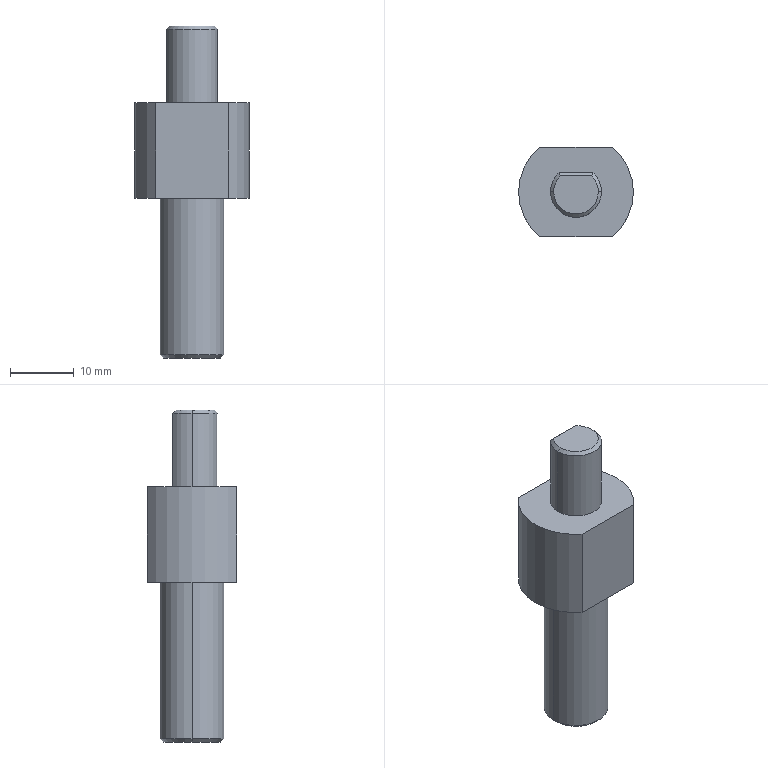Part | SolidWorks | features ICE 2, Chamfer 1, Extrusion 1 | 1 solid | 21 faces | box 18 x 14 x 52 mm | volume 5870 mm3 | cylinder 8 | plane 8 | cone 5 | commonest cylinder face diameters 8 x3 18 x3 10 x2
STEP:
#1=CARTESIAN_POINT('',(-4.5,0.,-52.));
#2=VERTEX_POINT('',#1);
#3=CARTESIAN_POINT('',(4.5,0.,-52.));
#4=VERTEX_POINT('',#3);
#5=CARTESIAN_POINT('',(0.,0.,-52.));
#6=DIRECTION('',(0.,0.,-1.));
#7=DIRECTION('',(-1.,0.,0.));
#8=AXIS2_PLACEMENT_3D('',#5,#6,#7);
#9=CIRCLE('',#8,4.5);
#10=EDGE_CURVE('',#2,#4,#9,.T.);
#11=ORIENTED_EDGE('',*,*,#10,.F.);
#12=CARTESIAN_POINT('',(-5.,0.,-51.5));
#13=VERTEX_POINT('',#12);
#14=CARTESIAN_POINT('',(-4.5,0.,-52.));
#15=DIRECTION('',(-0.7071,0.,0.7071));
#16=VECTOR('',#15,1000.);
#17=LINE('',#14,#16);
#18=EDGE_CURVE('',#2,#13,#17,.T.);
#19=ORIENTED_EDGE('',*,*,#18,.T.);
#20=CARTESIAN_POINT('',(5.,0.,-51.5));
#21=VERTEX_POINT('',#20);
#22=CARTESIAN_POINT('',(0.,0.,-51.5));
#23=DIRECTION('',(0.,0.,1.));
#24=DIRECTION('',(-1.,0.,0.));
#25=AXIS2_PLACEMENT_3D('',#22,#23,#24);
#26=CIRCLE('',#25,5.);
#27=EDGE_CURVE('',#21,#13,#26,.T.);
#28=ORIENTED_EDGE('',*,*,#27,.F.);
#29=CARTESIAN_POINT('',(4.5,0.,-52.));
#30=DIRECTION('',(0.7071,0.,0.7071));
#31=VECTOR('',#30,1000.);
#32=LINE('',#29,#31);
#33=EDGE_CURVE('',#4,#21,#32,.T.);
#34=ORIENTED_EDGE('',*,*,#33,.F.);
#35=EDGE_LOOP('',(#11,#19,#28,#34));
#36=FACE_OUTER_BOUND('',#35,.T.);
#37=CARTESIAN_POINT('',(0.,0.,-52.));
#38=DIRECTION('',(0.,0.,1.));
#39=DIRECTION('',(1.,0.,0.));
#40=AXIS2_PLACEMENT_3D('',#37,#38,#39);
#41=CONICAL_SURFACE('',#40,4.5,0.7854);
#42=ADVANCED_FACE('',(#36),#41,.T.);
#43=CARTESIAN_POINT('',(3.5,0.,0.));
#44=VERTEX_POINT('',#43);
#45=CARTESIAN_POINT('',(2.449,2.5,0.));
#46=VERTEX_POINT('',#45);
#47=CARTESIAN_POINT('',(0.,0.,0.));
#48=DIRECTION('',(0.,0.,1.));
#49=DIRECTION('',(1.,0.,0.));
#50=AXIS2_PLACEMENT_3D('',#47,#48,#49);
#51=CIRCLE('',#50,3.5);
#52=EDGE_CURVE('',#44,#46,#51,.T.);
#53=ORIENTED_EDGE('',*,*,#52,.F.);
#54=CARTESIAN_POINT('',(4.,0.,-0.5));
#55=VERTEX_POINT('',#54);
#56=CARTESIAN_POINT('',(3.5,0.,0.));
#57=DIRECTION('',(0.7071,0.,-0.7071));
#58=VECTOR('',#57,1000.);
#59=LINE('',#56,#58);
#60=EDGE_CURVE('',#44,#55,#59,.T.);
#61=ORIENTED_EDGE('',*,*,#60,.T.);
#62=CARTESIAN_POINT('',(2.646,3.,-0.5));
#63=VERTEX_POINT('',#62);
#64=CARTESIAN_POINT('',(0.,0.,-0.5));
#65=DIRECTION('',(0.,0.,-1.));
#66=DIRECTION('',(1.,0.,0.));
#67=AXIS2_PLACEMENT_3D('',#64,#65,#66);
#68=CIRCLE('',#67,4.);
#69=EDGE_CURVE('',#63,#55,#68,.T.);
#70=ORIENTED_EDGE('',*,*,#69,.F.);
#71=CARTESIAN_POINT('',(2.449,2.5,0.));
#72=CARTESIAN_POINT('',(2.517,2.666,-0.1662));
#73=CARTESIAN_POINT('',(2.583,2.833,-0.3329));
#74=CARTESIAN_POINT('',(2.646,3.,-0.5));
#75=B_SPLINE_CURVE_WITH_KNOTS('',3,(#71,#72,#73,#74),.UNSPECIFIED.,.F.,.F.,(4,4),(0.,0.0007338),.UNSPECIFIED.);
#76=EDGE_CURVE('',#46,#63,#75,.T.);
#77=ORIENTED_EDGE('',*,*,#76,.F.);
#78=EDGE_LOOP('',(#53,#61,#70,#77));
#79=FACE_OUTER_BOUND('',#78,.T.);
#80=CARTESIAN_POINT('',(0.,0.,0.));
#81=DIRECTION('',(0.,0.,-1.));
#82=DIRECTION('',(-1.,0.,0.));
#83=AXIS2_PLACEMENT_3D('',#80,#81,#82);
#84=CONICAL_SURFACE('',#83,3.5,0.7854);
#85=ADVANCED_FACE('',(#79),#84,.T.);
#86=ORIENTED_EDGE('',*,*,#60,.F.);
#87=CARTESIAN_POINT('',(-3.5,0.,0.));
#88=VERTEX_POINT('',#87);
#89=CARTESIAN_POINT('',(0.,0.,0.));
#90=DIRECTION('',(0.,0.,1.));
#91=DIRECTION('',(1.,0.,0.));
#92=AXIS2_PLACEMENT_3D('',#89,#90,#91);
#93=CIRCLE('',#92,3.5);
#94=EDGE_CURVE('',#88,#44,#93,.T.);
#95=ORIENTED_EDGE('',*,*,#94,.F.);
#96=CARTESIAN_POINT('',(-4.,0.,-0.5));
#97=VERTEX_POINT('',#96);
#98=CARTESIAN_POINT('',(-3.5,0.,0.));
#99=DIRECTION('',(-0.7071,0.,-0.7071));
#100=VECTOR('',#99,1000.);
#101=LINE('',#98,#100);
#102=EDGE_CURVE('',#88,#97,#101,.T.);
#103=ORIENTED_EDGE('',*,*,#102,.T.);
#104=CARTESIAN_POINT('',(0.,0.,-0.5));
#105=DIRECTION('',(0.,0.,-1.));
#106=DIRECTION('',(1.,0.,0.));
#107=AXIS2_PLACEMENT_3D('',#104,#105,#106);
#108=CIRCLE('',#107,4.);
#109=EDGE_CURVE('',#55,#97,#108,.T.);
#110=ORIENTED_EDGE('',*,*,#109,.F.);
#111=EDGE_LOOP('',(#86,#95,#103,#110));
#112=FACE_OUTER_BOUND('',#111,.T.);
#113=CARTESIAN_POINT('',(0.,0.,0.));
#114=DIRECTION('',(0.,0.,-1.));
#115=DIRECTION('',(-1.,0.,0.));
#116=AXIS2_PLACEMENT_3D('',#113,#114,#115);
#117=CONICAL_SURFACE('',#116,3.5,0.7854);
#118=ADVANCED_FACE('',(#112),#117,.T.);
#119=ORIENTED_EDGE('',*,*,#27,.T.);
#120=CARTESIAN_POINT('',(-5.,0.,-27.));
#121=VERTEX_POINT('',#120);
#122=CARTESIAN_POINT('',(-5.,0.,-52.));
#123=DIRECTION('',(0.,0.,1.));
#124=VECTOR('',#123,1000.);
#125=LINE('',#122,#124);
#126=EDGE_CURVE('',#13,#121,#125,.T.);
#127=ORIENTED_EDGE('',*,*,#126,.T.);
#128=CARTESIAN_POINT('',(5.,0.,-27.));
#129=VERTEX_POINT('',#128);
#130=CARTESIAN_POINT('',(0.,0.,-27.));
#131=DIRECTION('',(0.,0.,-1.));
#132=DIRECTION('',(-1.,0.,0.));
#133=AXIS2_PLACEMENT_3D('',#130,#131,#132);
#134=CIRCLE('',#133,5.);
#135=EDGE_CURVE('',#121,#129,#134,.T.);
#136=ORIENTED_EDGE('',*,*,#135,.T.);
#137=CARTESIAN_POINT('',(5.,0.,-52.));
#138=DIRECTION('',(0.,0.,1.));
#139=VECTOR('',#138,1000.);
#140=LINE('',#137,#139);
#141=EDGE_CURVE('',#21,#129,#140,.T.);
#142=ORIENTED_EDGE('',*,*,#141,.F.);
#143=EDGE_LOOP('',(#119,#127,#136,#142));
#144=FACE_OUTER_BOUND('',#143,.T.);
#145=CARTESIAN_POINT('',(0.,0.,-52.));
#146=DIRECTION('',(0.,0.,1.));
#147=DIRECTION('',(1.,0.,0.));
#148=AXIS2_PLACEMENT_3D('',#145,#146,#147);
#149=CYLINDRICAL_SURFACE('',#148,5.);
#150=ADVANCED_FACE('',(#144),#149,.T.);
#151=CARTESIAN_POINT('',(9.,0.,-27.));
#152=VERTEX_POINT('',#151);
#153=CARTESIAN_POINT('',(5.657,-7.,-27.));
#154=VERTEX_POINT('',#153);
#155=CARTESIAN_POINT('',(0.,0.,-27.));
#156=DIRECTION('',(0.,0.,-1.));
#157=DIRECTION('',(-1.,0.,0.));
#158=AXIS2_PLACEMENT_3D('',#155,#156,#157);
#159=CIRCLE('',#158,9.);
#160=EDGE_CURVE('',#152,#154,#159,.T.);
#161=ORIENTED_EDGE('',*,*,#160,.F.);
#162=CARTESIAN_POINT('',(9.,0.,-12.));
#163=VERTEX_POINT('',#162);
#164=CARTESIAN_POINT('',(9.,0.,-27.));
#165=DIRECTION('',(0.,0.,1.));
#166=VECTOR('',#165,1000.);
#167=LINE('',#164,#166);
#168=EDGE_CURVE('',#152,#163,#167,.T.);
#169=ORIENTED_EDGE('',*,*,#168,.T.);
#170=CARTESIAN_POINT('',(5.657,-7.,-12.));
#171=VERTEX_POINT('',#170);
#172=CARTESIAN_POINT('',(0.,0.,-12.));
#173=DIRECTION('',(0.,0.,-1.));
#174=DIRECTION('',(-1.,0.,0.));
#175=AXIS2_PLACEMENT_3D('',#172,#173,#174);
#176=CIRCLE('',#175,9.);
#177=EDGE_CURVE('',#163,#171,#176,.T.);
#178=ORIENTED_EDGE('',*,*,#177,.T.);
#179=CARTESIAN_POINT('',(5.657,-7.,-27.));
#180=DIRECTION('',(0.,0.,1.));
#181=VECTOR('',#180,1000.);
#182=LINE('',#179,#181);
#183=EDGE_CURVE('',#154,#171,#182,.T.);
#184=ORIENTED_EDGE('',*,*,#183,.F.);
#185=EDGE_LOOP('',(#161,#169,#178,#184));
#186=FACE_OUTER_BOUND('',#185,.T.);
#187=CARTESIAN_POINT('',(0.,0.,-27.));
#188=DIRECTION('',(0.,0.,1.));
#189=DIRECTION('',(1.,0.,0.));
#190=AXIS2_PLACEMENT_3D('',#187,#188,#189);
#191=CYLINDRICAL_SURFACE('',#190,9.);
#192=ADVANCED_FACE('',(#186),#191,.T.);
#193=CARTESIAN_POINT('',(-2.646,3.,-12.));
#194=VERTEX_POINT('',#193);
#195=CARTESIAN_POINT('',(-4.,0.,-12.));
#196=VERTEX_POINT('',#195);
#197=CARTESIAN_POINT('',(0.,0.,-12.));
#198=DIRECTION('',(0.,0.,1.));
#199=DIRECTION('',(1.,0.,0.));
#200=AXIS2_PLACEMENT_3D('',#197,#198,#199);
#201=CIRCLE('',#200,4.);
#202=EDGE_CURVE('',#194,#196,#201,.T.);
#203=ORIENTED_EDGE('',*,*,#202,.T.);
#204=CARTESIAN_POINT('',(-4.,0.,-12.));
#205=DIRECTION('',(0.,0.,1.));
#206=VECTOR('',#205,1000.);
#207=LINE('',#204,#206);
#208=EDGE_CURVE('',#196,#97,#207,.T.);
#209=ORIENTED_EDGE('',*,*,#208,.T.);
#210=CARTESIAN_POINT('',(-2.646,3.,-0.5));
#211=VERTEX_POINT('',#210);
#212=CARTESIAN_POINT('',(0.,0.,-0.5));
#213=DIRECTION('',(0.,0.,-1.));
#214=DIRECTION('',(1.,0.,0.));
#215=AXIS2_PLACEMENT_3D('',#212,#213,#214);
#216=CIRCLE('',#215,4.);
#217=EDGE_CURVE('',#97,#211,#216,.T.);
#218=ORIENTED_EDGE('',*,*,#217,.T.);
#219=CARTESIAN_POINT('',(-2.646,3.,-12.));
#220=DIRECTION('',(0.,0.,1.));
#221=VECTOR('',#220,1000.);
#222=LINE('',#219,#221);
#223=EDGE_CURVE('',#194,#211,#222,.T.);
#224=ORIENTED_EDGE('',*,*,#223,.F.);
#225=EDGE_LOOP('',(#203,#209,#218,#224));
#226=FACE_OUTER_BOUND('',#225,.T.);
#227=CARTESIAN_POINT('',(0.,0.,-12.));
#228=DIRECTION('',(0.,0.,1.));
#229=DIRECTION('',(1.,0.,0.));
#230=AXIS2_PLACEMENT_3D('',#227,#228,#229);
#231=CYLINDRICAL_SURFACE('',#230,4.);
#232=ADVANCED_FACE('',(#226),#231,.T.);
#233=ORIENTED_EDGE('',*,*,#208,.F.);
#234=CARTESIAN_POINT('',(4.,0.,-12.));
#235=VERTEX_POINT('',#234);
#236=CARTESIAN_POINT('',(0.,0.,-12.));
#237=DIRECTION('',(0.,0.,1.));
#238=DIRECTION('',(1.,0.,0.));
#239=AXIS2_PLACEMENT_3D('',#236,#237,#238);
#240=CIRCLE('',#239,4.);
#241=EDGE_CURVE('',#196,#235,#240,.T.);
#242=ORIENTED_EDGE('',*,*,#241,.T.);
#243=CARTESIAN_POINT('',(4.,0.,-12.));
#244=DIRECTION('',(0.,0.,1.));
#245=VECTOR('',#244,1000.);
#246=LINE('',#243,#245);
#247=EDGE_CURVE('',#235,#55,#246,.T.);
#248=ORIENTED_EDGE('',*,*,#247,.T.);
#249=ORIENTED_EDGE('',*,*,#109,.T.);
#250=EDGE_LOOP('',(#233,#242,#248,#249));
#251=FACE_OUTER_BOUND('',#250,.T.);
#252=CARTESIAN_POINT('',(0.,0.,-12.));
#253=DIRECTION('',(0.,0.,1.));
#254=DIRECTION('',(1.,0.,0.));
#255=AXIS2_PLACEMENT_3D('',#252,#253,#254);
#256=CYLINDRICAL_SURFACE('',#255,4.);
#257=ADVANCED_FACE('',(#251),#256,.T.);
#258=ORIENTED_EDGE('',*,*,#247,.F.);
#259=CARTESIAN_POINT('',(2.646,3.,-12.));
#260=VERTEX_POINT('',#259);
#261=CARTESIAN_POINT('',(0.,0.,-12.));
#262=DIRECTION('',(0.,0.,1.));
#263=DIRECTION('',(1.,0.,0.));
#264=AXIS2_PLACEMENT_3D('',#261,#262,#263);
#265=CIRCLE('',#264,4.);
#266=EDGE_CURVE('',#235,#260,#265,.T.);
#267=ORIENTED_EDGE('',*,*,#266,.T.);
#268=CARTESIAN_POINT('',(2.646,3.,-12.));
#269=DIRECTION('',(0.,0.,1.));
#270=VECTOR('',#269,1000.);
#271=LINE('',#268,#270);
#272=EDGE_CURVE('',#260,#63,#271,.T.);
#273=ORIENTED_EDGE('',*,*,#272,.T.);
#274=ORIENTED_EDGE('',*,*,#69,.T.);
#275=EDGE_LOOP('',(#258,#267,#273,#274));
#276=FACE_OUTER_BOUND('',#275,.T.);
#277=CARTESIAN_POINT('',(0.,0.,-12.));
#278=DIRECTION('',(0.,0.,1.));
#279=DIRECTION('',(1.,0.,0.));
#280=AXIS2_PLACEMENT_3D('',#277,#278,#279);
#281=CYLINDRICAL_SURFACE('',#280,4.);
#282=ADVANCED_FACE('',(#276),#281,.T.);
#283=ORIENTED_EDGE('',*,*,#223,.T.);
#284=CARTESIAN_POINT('',(2.646,3.,-0.5));
#285=DIRECTION('',(1.,0.,0.));
#286=VECTOR('',#285,1000.);
#287=LINE('',#284,#286);
#288=EDGE_CURVE('',#211,#63,#287,.T.);
#289=ORIENTED_EDGE('',*,*,#288,.T.);
#290=ORIENTED_EDGE('',*,*,#272,.F.);
#291=CARTESIAN_POINT('',(0.,3.,-12.));
#292=DIRECTION('',(1.,0.,0.));
#293=VECTOR('',#292,1000.);
#294=LINE('',#291,#293);
#295=EDGE_CURVE('',#194,#260,#294,.T.);
#296=ORIENTED_EDGE('',*,*,#295,.F.);
#297=EDGE_LOOP('',(#283,#289,#290,#296));
#298=FACE_OUTER_BOUND('',#297,.T.);
#299=CARTESIAN_POINT('',(0.,3.,-12.));
#300=DIRECTION('',(0.,-1.,0.));
#301=DIRECTION('',(0.,0.,-1.));
#302=AXIS2_PLACEMENT_3D('',#299,#300,#301);
#303=PLANE('',#302);
#304=ADVANCED_FACE('',(#298),#303,.F.);
#305=CARTESIAN_POINT('',(-2.449,2.5,0.));
#306=VERTEX_POINT('',#305);
#307=CARTESIAN_POINT('',(0.,0.,0.));
#308=DIRECTION('',(0.,0.,1.));
#309=DIRECTION('',(1.,0.,0.));
#310=AXIS2_PLACEMENT_3D('',#307,#308,#309);
#311=CIRCLE('',#310,3.5);
#312=EDGE_CURVE('',#306,#88,#311,.T.);
#313=ORIENTED_EDGE('',*,*,#312,.T.);
#314=ORIENTED_EDGE('',*,*,#94,.T.);
#315=ORIENTED_EDGE('',*,*,#52,.T.);
#316=CARTESIAN_POINT('',(-2.646,2.5,0.));
#317=DIRECTION('',(-1.,0.,0.));
#318=VECTOR('',#317,1000.);
#319=LINE('',#316,#318);
#320=EDGE_CURVE('',#46,#306,#319,.T.);
#321=ORIENTED_EDGE('',*,*,#320,.T.);
#322=EDGE_LOOP('',(#313,#314,#315,#321));
#323=FACE_OUTER_BOUND('',#322,.T.);
#324=CARTESIAN_POINT('',(0.,0.,0.));
#325=DIRECTION('',(0.,0.,1.));
#326=DIRECTION('',(1.,0.,0.));
#327=AXIS2_PLACEMENT_3D('',#324,#325,#326);
#328=PLANE('',#327);
#329=ADVANCED_FACE('',(#323),#328,.T.);
#330=CARTESIAN_POINT('',(5.657,7.,-12.));
#331=VERTEX_POINT('',#330);
#332=CARTESIAN_POINT('',(-5.657,7.,-12.));
#333=VERTEX_POINT('',#332);
#334=CARTESIAN_POINT('',(0.,7.,-12.));
#335=DIRECTION('',(-1.,0.,0.));
#336=VECTOR('',#335,1000.);
#337=LINE('',#334,#336);
#338=EDGE_CURVE('',#331,#333,#337,.T.);
#339=ORIENTED_EDGE('',*,*,#338,.F.);
#340=CARTESIAN_POINT('',(5.657,7.,-27.));
#341=VERTEX_POINT('',#340);
#342=CARTESIAN_POINT('',(5.657,7.,-27.));
#343=DIRECTION('',(0.,0.,1.));
#344=VECTOR('',#343,1000.);
#345=LINE('',#342,#344);
#346=EDGE_CURVE('',#341,#331,#345,.T.);
#347=ORIENTED_EDGE('',*,*,#346,.F.);
#348=CARTESIAN_POINT('',(-5.657,7.,-27.));
#349=VERTEX_POINT('',#348);
#350=CARTESIAN_POINT('',(0.,7.,-27.));
#351=DIRECTION('',(-1.,0.,0.));
#352=VECTOR('',#351,1000.);
#353=LINE('',#350,#352);
#354=EDGE_CURVE('',#341,#349,#353,.T.);
#355=ORIENTED_EDGE('',*,*,#354,.T.);
#356=CARTESIAN_POINT('',(-5.657,7.,-27.));
#357=DIRECTION('',(0.,0.,1.));
#358=VECTOR('',#357,1000.);
#359=LINE('',#356,#358);
#360=EDGE_CURVE('',#349,#333,#359,.T.);
#361=ORIENTED_EDGE('',*,*,#360,.T.);
#362=EDGE_LOOP('',(#339,#347,#355,#361));
#363=FACE_OUTER_BOUND('',#362,.T.);
#364=CARTESIAN_POINT('',(0.,7.,-27.));
#365=DIRECTION('',(0.,1.,0.));
#366=DIRECTION('',(0.,0.,1.));
#367=AXIS2_PLACEMENT_3D('',#364,#365,#366);
#368=PLANE('',#367);
#369=ADVANCED_FACE('',(#363),#368,.T.);
#370=ORIENTED_EDGE('',*,*,#168,.F.);
#371=CARTESIAN_POINT('',(0.,0.,-27.));
#372=DIRECTION('',(0.,0.,-1.));
#373=DIRECTION('',(-1.,0.,0.));
#374=AXIS2_PLACEMENT_3D('',#371,#372,#373);
#375=CIRCLE('',#374,9.);
#376=EDGE_CURVE('',#341,#152,#375,.T.);
#377=ORIENTED_EDGE('',*,*,#376,.F.);
#378=ORIENTED_EDGE('',*,*,#346,.T.);
#379=CARTESIAN_POINT('',(0.,0.,-12.));
#380=DIRECTION('',(0.,0.,-1.));
#381=DIRECTION('',(-1.,0.,0.));
#382=AXIS2_PLACEMENT_3D('',#379,#380,#381);
#383=CIRCLE('',#382,9.);
#384=EDGE_CURVE('',#331,#163,#383,.T.);
#385=ORIENTED_EDGE('',*,*,#384,.T.);
#386=EDGE_LOOP('',(#370,#377,#378,#385));
#387=FACE_OUTER_BOUND('',#386,.T.);
#388=CARTESIAN_POINT('',(0.,0.,-27.));
#389=DIRECTION('',(0.,0.,1.));
#390=DIRECTION('',(1.,0.,0.));
#391=AXIS2_PLACEMENT_3D('',#388,#389,#390);
#392=CYLINDRICAL_SURFACE('',#391,9.);
#393=ADVANCED_FACE('',(#387),#392,.T.);
#394=CARTESIAN_POINT('',(-5.657,-7.,-12.));
#395=VERTEX_POINT('',#394);
#396=CARTESIAN_POINT('',(0.,-7.,-12.));
#397=DIRECTION('',(-1.,0.,0.));
#398=VECTOR('',#397,1000.);
#399=LINE('',#396,#398);
#400=EDGE_CURVE('',#171,#395,#399,.T.);
#401=ORIENTED_EDGE('',*,*,#400,.T.);
#402=CARTESIAN_POINT('',(-5.657,-7.,-27.));
#403=VERTEX_POINT('',#402);
#404=CARTESIAN_POINT('',(-5.657,-7.,-27.));
#405=DIRECTION('',(0.,0.,1.));
#406=VECTOR('',#405,1000.);
#407=LINE('',#404,#406);
#408=EDGE_CURVE('',#403,#395,#407,.T.);
#409=ORIENTED_EDGE('',*,*,#408,.F.);
#410=CARTESIAN_POINT('',(0.,-7.,-27.));
#411=DIRECTION('',(-1.,0.,0.));
#412=VECTOR('',#411,1000.);
#413=LINE('',#410,#412);
#414=EDGE_CURVE('',#154,#403,#413,.T.);
#415=ORIENTED_EDGE('',*,*,#414,.F.);
#416=ORIENTED_EDGE('',*,*,#183,.T.);
#417=EDGE_LOOP('',(#401,#409,#415,#416));
#418=FACE_OUTER_BOUND('',#417,.T.);
#419=CARTESIAN_POINT('',(0.,-7.,-27.));
#420=DIRECTION('',(0.,1.,0.));
#421=DIRECTION('',(0.,0.,1.));
#422=AXIS2_PLACEMENT_3D('',#419,#420,#421);
#423=PLANE('',#422);
#424=ADVANCED_FACE('',(#418),#423,.F.);
#425=CARTESIAN_POINT('',(0.,0.,-12.));
#426=DIRECTION('',(0.,0.,-1.));
#427=DIRECTION('',(-1.,0.,0.));
#428=AXIS2_PLACEMENT_3D('',#425,#426,#427);
#429=CIRCLE('',#428,9.);
#430=EDGE_CURVE('',#395,#333,#429,.T.);
#431=ORIENTED_EDGE('',*,*,#430,.T.);
#432=ORIENTED_EDGE('',*,*,#360,.F.);
#433=CARTESIAN_POINT('',(0.,0.,-27.));
#434=DIRECTION('',(0.,0.,-1.));
#435=DIRECTION('',(-1.,0.,0.));
#436=AXIS2_PLACEMENT_3D('',#433,#434,#435);
#437=CIRCLE('',#436,9.);
#438=EDGE_CURVE('',#403,#349,#437,.T.);
#439=ORIENTED_EDGE('',*,*,#438,.F.);
#440=ORIENTED_EDGE('',*,*,#408,.T.);
#441=EDGE_LOOP('',(#431,#432,#439,#440));
#442=FACE_OUTER_BOUND('',#441,.T.);
#443=CARTESIAN_POINT('',(0.,0.,-27.));
#444=DIRECTION('',(0.,0.,1.));
#445=DIRECTION('',(1.,0.,0.));
#446=AXIS2_PLACEMENT_3D('',#443,#444,#445);
#447=CYLINDRICAL_SURFACE('',#446,9.);
#448=ADVANCED_FACE('',(#442),#447,.T.);
#449=CARTESIAN_POINT('',(0.,0.,-27.));
#450=DIRECTION('',(0.,0.,-1.));
#451=DIRECTION('',(-1.,0.,0.));
#452=AXIS2_PLACEMENT_3D('',#449,#450,#451);
#453=CIRCLE('',#452,5.);
#454=EDGE_CURVE('',#129,#121,#453,.T.);
#455=ORIENTED_EDGE('',*,*,#454,.F.);
#456=ORIENTED_EDGE('',*,*,#135,.F.);
#457=EDGE_LOOP('',(#455,#456));
#458=FACE_BOUND('',#457,.T.);
#459=ORIENTED_EDGE('',*,*,#354,.F.);
#460=ORIENTED_EDGE('',*,*,#376,.T.);
#461=ORIENTED_EDGE('',*,*,#160,.T.);
#462=ORIENTED_EDGE('',*,*,#414,.T.);
#463=ORIENTED_EDGE('',*,*,#438,.T.);
#464=EDGE_LOOP('',(#459,#460,#461,#462,#463));
#465=FACE_OUTER_BOUND('',#464,.T.);
#466=CARTESIAN_POINT('',(0.,0.,-27.));
#467=DIRECTION('',(0.,0.,-1.));
#468=DIRECTION('',(-1.,0.,0.));
#469=AXIS2_PLACEMENT_3D('',#466,#467,#468);
#470=PLANE('',#469);
#471=ADVANCED_FACE('',(#458,#465),#470,.T.);
#472=ORIENTED_EDGE('',*,*,#202,.F.);
#473=ORIENTED_EDGE('',*,*,#295,.T.);
#474=ORIENTED_EDGE('',*,*,#266,.F.);
#475=ORIENTED_EDGE('',*,*,#241,.F.);
#476=EDGE_LOOP('',(#472,#473,#474,#475));
#477=FACE_BOUND('',#476,.T.);
#478=ORIENTED_EDGE('',*,*,#338,.T.);
#479=ORIENTED_EDGE('',*,*,#430,.F.);
#480=ORIENTED_EDGE('',*,*,#400,.F.);
#481=ORIENTED_EDGE('',*,*,#177,.F.);
#482=ORIENTED_EDGE('',*,*,#384,.F.);
#483=EDGE_LOOP('',(#478,#479,#480,#481,#482));
#484=FACE_OUTER_BOUND('',#483,.T.);
#485=CARTESIAN_POINT('',(0.,0.,-12.));
#486=DIRECTION('',(0.,0.,-1.));
#487=DIRECTION('',(-1.,0.,0.));
#488=AXIS2_PLACEMENT_3D('',#485,#486,#487);
#489=PLANE('',#488);
#490=ADVANCED_FACE('',(#477,#484),#489,.F.);
#491=ORIENTED_EDGE('',*,*,#126,.F.);
#492=CARTESIAN_POINT('',(0.,0.,-51.5));
#493=DIRECTION('',(0.,0.,1.));
#494=DIRECTION('',(-1.,0.,0.));
#495=AXIS2_PLACEMENT_3D('',#492,#493,#494);
#496=CIRCLE('',#495,5.);
#497=EDGE_CURVE('',#13,#21,#496,.T.);
#498=ORIENTED_EDGE('',*,*,#497,.T.);
#499=ORIENTED_EDGE('',*,*,#141,.T.);
#500=ORIENTED_EDGE('',*,*,#454,.T.);
#501=EDGE_LOOP('',(#491,#498,#499,#500));
#502=FACE_OUTER_BOUND('',#501,.T.);
#503=CARTESIAN_POINT('',(0.,0.,-52.));
#504=DIRECTION('',(0.,0.,1.));
#505=DIRECTION('',(1.,0.,0.));
#506=AXIS2_PLACEMENT_3D('',#503,#504,#505);
#507=CYLINDRICAL_SURFACE('',#506,5.);
#508=ADVANCED_FACE('',(#502),#507,.T.);
#509=CARTESIAN_POINT('',(0.,0.,-52.));
#510=DIRECTION('',(0.,0.,-1.));
#511=DIRECTION('',(-1.,0.,0.));
#512=AXIS2_PLACEMENT_3D('',#509,#510,#511);
#513=CIRCLE('',#512,4.5);
#514=EDGE_CURVE('',#4,#2,#513,.T.);
#515=ORIENTED_EDGE('',*,*,#514,.T.);
#516=ORIENTED_EDGE('',*,*,#10,.T.);
#517=EDGE_LOOP('',(#515,#516));
#518=FACE_OUTER_BOUND('',#517,.T.);
#519=CARTESIAN_POINT('',(0.,0.,-52.));
#520=DIRECTION('',(0.,0.,-1.));
#521=DIRECTION('',(-1.,0.,0.));
#522=AXIS2_PLACEMENT_3D('',#519,#520,#521);
#523=PLANE('',#522);
#524=ADVANCED_FACE('',(#518),#523,.T.);
#525=ORIENTED_EDGE('',*,*,#102,.F.);
#526=ORIENTED_EDGE('',*,*,#312,.F.);
#527=CARTESIAN_POINT('',(-2.646,3.,-0.5));
#528=CARTESIAN_POINT('',(-2.583,2.833,-0.3329));
#529=CARTESIAN_POINT('',(-2.517,2.666,-0.1662));
#530=CARTESIAN_POINT('',(-2.449,2.5,0.));
#531=B_SPLINE_CURVE_WITH_KNOTS('',3,(#527,#528,#529,#530),.UNSPECIFIED.,.F.,.F.,(4,4),(0.,0.0007338),.UNSPECIFIED.);
#532=EDGE_CURVE('',#211,#306,#531,.T.);
#533=ORIENTED_EDGE('',*,*,#532,.F.);
#534=ORIENTED_EDGE('',*,*,#217,.F.);
#535=EDGE_LOOP('',(#525,#526,#533,#534));
#536=FACE_OUTER_BOUND('',#535,.T.);
#537=CARTESIAN_POINT('',(0.,0.,0.));
#538=DIRECTION('',(0.,0.,-1.));
#539=DIRECTION('',(-1.,0.,0.));
#540=AXIS2_PLACEMENT_3D('',#537,#538,#539);
#541=CONICAL_SURFACE('',#540,3.5,0.7854);
#542=ADVANCED_FACE('',(#536),#541,.T.);
#543=ORIENTED_EDGE('',*,*,#532,.T.);
#544=ORIENTED_EDGE('',*,*,#320,.F.);
#545=ORIENTED_EDGE('',*,*,#76,.T.);
#546=ORIENTED_EDGE('',*,*,#288,.F.);
#547=EDGE_LOOP('',(#543,#544,#545,#546));
#548=FACE_OUTER_BOUND('',#547,.T.);
#549=CARTESIAN_POINT('',(0.,3.,-0.5));
#550=DIRECTION('',(0.,0.7071,0.7071));
#551=DIRECTION('',(-1.,0.,0.));
#552=AXIS2_PLACEMENT_3D('',#549,#550,#551);
#553=PLANE('',#552);
#554=ADVANCED_FACE('',(#548),#553,.T.);
#555=ORIENTED_EDGE('',*,*,#18,.F.);
#556=ORIENTED_EDGE('',*,*,#514,.F.);
#557=ORIENTED_EDGE('',*,*,#33,.T.);
#558=ORIENTED_EDGE('',*,*,#497,.F.);
#559=EDGE_LOOP('',(#555,#556,#557,#558));
#560=FACE_OUTER_BOUND('',#559,.T.);
#561=CARTESIAN_POINT('',(0.,0.,-52.));
#562=DIRECTION('',(0.,0.,1.));
#563=DIRECTION('',(1.,0.,0.));
#564=AXIS2_PLACEMENT_3D('',#561,#562,#563);
#565=CONICAL_SURFACE('',#564,4.5,0.7854);
#566=ADVANCED_FACE('',(#560),#565,.T.);
#567=CLOSED_SHELL('',(#42,#85,#118,#150,#192,#232,#257,#282,#304,#329,#369,#393,#424,#448,#471,#490,#508,#524,#542,#554,#566));
#568=MANIFOLD_SOLID_BREP('',#567);
#569=CARTESIAN_POINT('',(0.,0.,0.));
#570=DIRECTION('',(0.,0.,1.));
#571=DIRECTION('',(1.,0.,0.));
#572=AXIS2_PLACEMENT_3D('',#569,#570,#571);
#573=(LENGTH_UNIT()NAMED_UNIT(*)SI_UNIT(.MILLI.,.METRE.));
#574=UNCERTAINTY_MEASURE_WITH_UNIT(LENGTH_MEASURE(0.00001),#573,'','');
#575=(NAMED_UNIT(*)PLANE_ANGLE_UNIT()SI_UNIT($,.RADIAN.));
#576=(NAMED_UNIT(*)SI_UNIT($,.STERADIAN.)SOLID_ANGLE_UNIT());
#577=(GEOMETRIC_REPRESENTATION_CONTEXT(3)GLOBAL_UNCERTAINTY_ASSIGNED_CONTEXT((#574))GLOBAL_UNIT_ASSIGNED_CONTEXT((#573,#575,#576))REPRESENTATION_CONTEXT('',''));
#578=ADVANCED_BREP_SHAPE_REPRESENTATION('',(#568,#572),#577);